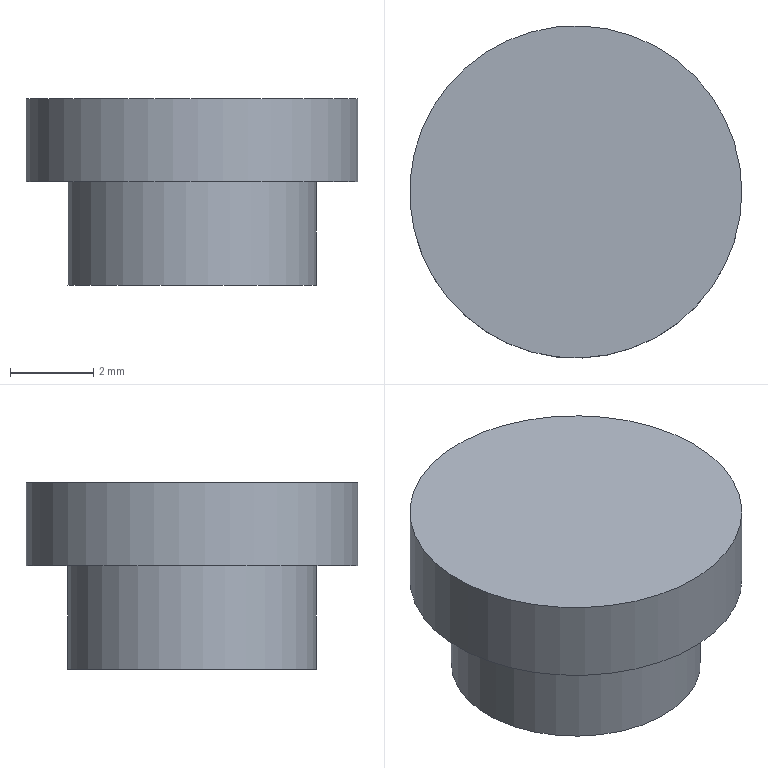Part | NX | features CYLINDER 2, DATUM_CSYS 1 | 1 solid | 5 faces | box 8 x 8 x 4.5 mm | volume 171.217 mm3 | plane 3 | cylinder 2 | commonest cylinder face diameters 6 x1 8 x1
STEP:
#1=CARTESIAN_POINT('',(3.,0.,0.));
#2=VERTEX_POINT('',#1);
#3=CARTESIAN_POINT('',(0.,0.,0.));
#4=DIRECTION('',(0.,0.,1.));
#5=DIRECTION('',(1.,0.,0.));
#6=AXIS2_PLACEMENT_3D('',#3,#4,#5);
#7=CIRCLE('',#6,3.);
#8=EDGE_CURVE('',#2,#2,#7,.T.);
#9=ORIENTED_EDGE('',*,*,#8,.F.);
#10=EDGE_LOOP('',(#9));
#11=FACE_BOUND('',#10,.T.);
#12=CARTESIAN_POINT('',(0.,0.,0.));
#13=DIRECTION('',(0.,0.,-1.));
#14=DIRECTION('',(-1.,0.,0.));
#15=AXIS2_PLACEMENT_3D('',#12,#13,#14);
#16=PLANE('',#15);
#17=ADVANCED_FACE('',(#11),#16,.T.);
#18=CARTESIAN_POINT('',(3.,0.,2.5));
#19=VERTEX_POINT('',#18);
#20=CARTESIAN_POINT('',(0.,0.,2.5));
#21=DIRECTION('',(0.,0.,-1.));
#22=DIRECTION('',(1.,0.,0.));
#23=AXIS2_PLACEMENT_3D('',#20,#21,#22);
#24=CIRCLE('',#23,3.);
#25=EDGE_CURVE('',#19,#19,#24,.T.);
#26=ORIENTED_EDGE('',*,*,#25,.T.);
#27=EDGE_LOOP('',(#26));
#28=FACE_BOUND('',#27,.T.);
#29=ORIENTED_EDGE('',*,*,#8,.T.);
#30=EDGE_LOOP('',(#29));
#31=FACE_BOUND('',#30,.T.);
#32=CARTESIAN_POINT('',(0.,0.,0.));
#33=DIRECTION('',(0.,0.,1.));
#34=DIRECTION('',(1.,0.,0.));
#35=AXIS2_PLACEMENT_3D('',#32,#33,#34);
#36=CYLINDRICAL_SURFACE('',#35,3.);
#37=ADVANCED_FACE('',(#28,#31),#36,.T.);
#38=CARTESIAN_POINT('',(4.,0.,4.5));
#39=VERTEX_POINT('',#38);
#40=CARTESIAN_POINT('',(0.,0.,4.5));
#41=DIRECTION('',(0.,0.,-1.));
#42=DIRECTION('',(1.,0.,0.));
#43=AXIS2_PLACEMENT_3D('',#40,#41,#42);
#44=CIRCLE('',#43,4.);
#45=EDGE_CURVE('',#39,#39,#44,.T.);
#46=ORIENTED_EDGE('',*,*,#45,.F.);
#47=EDGE_LOOP('',(#46));
#48=FACE_BOUND('',#47,.T.);
#49=CARTESIAN_POINT('',(0.,0.,4.5));
#50=DIRECTION('',(0.,0.,1.));
#51=DIRECTION('',(1.,0.,0.));
#52=AXIS2_PLACEMENT_3D('',#49,#50,#51);
#53=PLANE('',#52);
#54=ADVANCED_FACE('',(#48),#53,.T.);
#55=ORIENTED_EDGE('',*,*,#25,.F.);
#56=EDGE_LOOP('',(#55));
#57=FACE_BOUND('',#56,.T.);
#58=CARTESIAN_POINT('',(4.,0.,2.5));
#59=VERTEX_POINT('',#58);
#60=CARTESIAN_POINT('',(0.,0.,2.5));
#61=DIRECTION('',(0.,0.,1.));
#62=DIRECTION('',(1.,0.,0.));
#63=AXIS2_PLACEMENT_3D('',#60,#61,#62);
#64=CIRCLE('',#63,4.);
#65=EDGE_CURVE('',#59,#59,#64,.T.);
#66=ORIENTED_EDGE('',*,*,#65,.F.);
#67=EDGE_LOOP('',(#66));
#68=FACE_BOUND('',#67,.T.);
#69=CARTESIAN_POINT('',(0.,0.,2.5));
#70=DIRECTION('',(0.,0.,-1.));
#71=DIRECTION('',(-1.,0.,0.));
#72=AXIS2_PLACEMENT_3D('',#69,#70,#71);
#73=PLANE('',#72);
#74=ADVANCED_FACE('',(#57,#68),#73,.T.);
#75=ORIENTED_EDGE('',*,*,#45,.T.);
#76=EDGE_LOOP('',(#75));
#77=FACE_BOUND('',#76,.T.);
#78=ORIENTED_EDGE('',*,*,#65,.T.);
#79=EDGE_LOOP('',(#78));
#80=FACE_BOUND('',#79,.T.);
#81=CARTESIAN_POINT('',(0.,0.,2.5));
#82=DIRECTION('',(0.,0.,1.));
#83=DIRECTION('',(1.,0.,0.));
#84=AXIS2_PLACEMENT_3D('',#81,#82,#83);
#85=CYLINDRICAL_SURFACE('',#84,4.);
#86=ADVANCED_FACE('',(#77,#80),#85,.T.);
#87=CLOSED_SHELL('',(#17,#37,#54,#74,#86));
#88=MANIFOLD_SOLID_BREP('',#87);
#89=(LENGTH_UNIT()NAMED_UNIT(*)SI_UNIT(.MILLI.,.METRE.));
#90=UNCERTAINTY_MEASURE_WITH_UNIT(LENGTH_MEASURE(0.00001),#89,'','');
#91=(NAMED_UNIT(*)PLANE_ANGLE_UNIT()SI_UNIT($,.RADIAN.));
#92=(NAMED_UNIT(*)SI_UNIT($,.STERADIAN.)SOLID_ANGLE_UNIT());
#93=(GEOMETRIC_REPRESENTATION_CONTEXT(3)GLOBAL_UNCERTAINTY_ASSIGNED_CONTEXT((#90))GLOBAL_UNIT_ASSIGNED_CONTEXT((#89,#91,#92))REPRESENTATION_CONTEXT('',''));
#94=ADVANCED_BREP_SHAPE_REPRESENTATION('',(#88),#93);